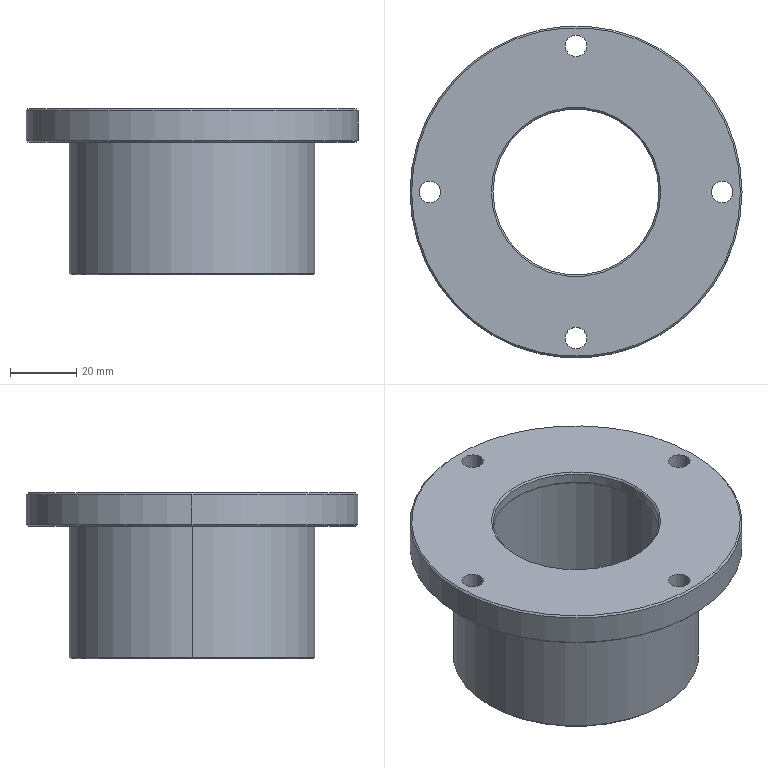Part | STEP file | 2087 Bag feed material shaft A | 1 solid | 48 faces | box 100 x 100 x 50 mm | volume 131531 mm3 | cylinder 24 | cone 20 | plane 4 | commonest cylinder face diameters 3.3 x8 6.5 x8 50 x2 55 x2 74 x2 100 x2